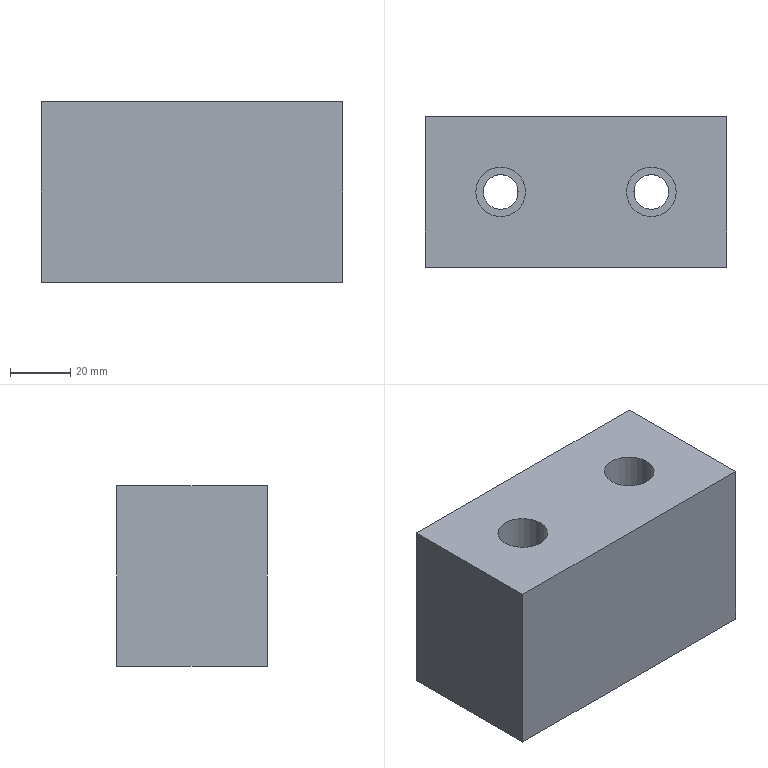Part | NX | features solid 2 | 1 solid | 12 faces | box 100 x 50 x 60 mm | volume 284237 mm3 | plane 8 | cylinder 4 | commonest cylinder face diameters 11.5 x2 16.5 x2
STEP:
#1=CARTESIAN_POINT('',(-1315.,-382.5,-70.));
#2=VERTEX_POINT('',#1);
#3=CARTESIAN_POINT('',(-1315.,-382.5,-130.));
#4=VERTEX_POINT('',#3);
#5=CARTESIAN_POINT('',(-1315.,-382.5,-140.));
#6=DIRECTION('',(0.,0.,1.));
#7=VECTOR('',#6,1000.);
#8=LINE('',#5,#7);
#9=EDGE_CURVE('',#2,#4,#8,.F.);
#10=ORIENTED_EDGE('',*,*,#9,.F.);
#11=CARTESIAN_POINT('',(-1415.,-382.5,-70.));
#12=VERTEX_POINT('',#11);
#13=CARTESIAN_POINT('',(-1325.,-382.5,-70.));
#14=DIRECTION('',(-1.,0.,0.));
#15=VECTOR('',#14,1000.);
#16=LINE('',#13,#15);
#17=EDGE_CURVE('',#2,#12,#16,.T.);
#18=ORIENTED_EDGE('',*,*,#17,.T.);
#19=CARTESIAN_POINT('',(-1415.,-382.5,-130.));
#20=VERTEX_POINT('',#19);
#21=CARTESIAN_POINT('',(-1415.,-382.5,-140.));
#22=DIRECTION('',(0.,0.,-1.));
#23=VECTOR('',#22,1000.);
#24=LINE('',#21,#23);
#25=EDGE_CURVE('',#12,#20,#24,.T.);
#26=ORIENTED_EDGE('',*,*,#25,.T.);
#27=CARTESIAN_POINT('',(-1325.,-382.5,-130.));
#28=DIRECTION('',(-1.,0.,0.));
#29=VECTOR('',#28,1000.);
#30=LINE('',#27,#29);
#31=EDGE_CURVE('',#4,#20,#30,.T.);
#32=ORIENTED_EDGE('',*,*,#31,.F.);
#33=EDGE_LOOP('',(#10,#18,#26,#32));
#34=FACE_BOUND('',#33,.T.);
#35=CARTESIAN_POINT('',(-1325.,-382.5,-140.));
#36=DIRECTION('',(0.,-1.,0.));
#37=DIRECTION('',(-1.,0.,0.));
#38=AXIS2_PLACEMENT_3D('',#35,#36,#37);
#39=PLANE('',#38);
#40=ADVANCED_FACE('',(#34),#39,.T.);
#41=ORIENTED_EDGE('',*,*,#25,.F.);
#42=CARTESIAN_POINT('',(-1415.,-332.5,-70.));
#43=VERTEX_POINT('',#42);
#44=CARTESIAN_POINT('',(-1415.,-367.5,-70.));
#45=DIRECTION('',(0.,1.,0.));
#46=VECTOR('',#45,1000.);
#47=LINE('',#44,#46);
#48=EDGE_CURVE('',#12,#43,#47,.T.);
#49=ORIENTED_EDGE('',*,*,#48,.T.);
#50=CARTESIAN_POINT('',(-1415.,-332.5,-130.));
#51=VERTEX_POINT('',#50);
#52=CARTESIAN_POINT('',(-1415.,-332.5,-140.));
#53=DIRECTION('',(0.,0.,1.));
#54=VECTOR('',#53,1000.);
#55=LINE('',#52,#54);
#56=EDGE_CURVE('',#43,#51,#55,.F.);
#57=ORIENTED_EDGE('',*,*,#56,.T.);
#58=CARTESIAN_POINT('',(-1415.,-367.5,-130.));
#59=DIRECTION('',(0.,1.,0.));
#60=VECTOR('',#59,1000.);
#61=LINE('',#58,#60);
#62=EDGE_CURVE('',#20,#51,#61,.T.);
#63=ORIENTED_EDGE('',*,*,#62,.F.);
#64=EDGE_LOOP('',(#41,#49,#57,#63));
#65=FACE_BOUND('',#64,.T.);
#66=CARTESIAN_POINT('',(-1415.,-367.5,-140.));
#67=DIRECTION('',(-1.,0.,0.));
#68=DIRECTION('',(0.,1.,0.));
#69=AXIS2_PLACEMENT_3D('',#66,#67,#68);
#70=PLANE('',#69);
#71=ADVANCED_FACE('',(#65),#70,.T.);
#72=ORIENTED_EDGE('',*,*,#56,.F.);
#73=CARTESIAN_POINT('',(-1315.,-332.5,-70.));
#74=VERTEX_POINT('',#73);
#75=CARTESIAN_POINT('',(-1325.,-332.5,-70.));
#76=DIRECTION('',(1.,0.,0.));
#77=VECTOR('',#76,1000.);
#78=LINE('',#75,#77);
#79=EDGE_CURVE('',#74,#43,#78,.F.);
#80=ORIENTED_EDGE('',*,*,#79,.F.);
#81=CARTESIAN_POINT('',(-1315.,-332.5,-130.));
#82=VERTEX_POINT('',#81);
#83=CARTESIAN_POINT('',(-1315.,-332.5,-140.));
#84=DIRECTION('',(0.,0.,-1.));
#85=VECTOR('',#84,1000.);
#86=LINE('',#83,#85);
#87=EDGE_CURVE('',#74,#82,#86,.T.);
#88=ORIENTED_EDGE('',*,*,#87,.T.);
#89=CARTESIAN_POINT('',(-1325.,-332.5,-130.));
#90=DIRECTION('',(1.,0.,0.));
#91=VECTOR('',#90,1000.);
#92=LINE('',#89,#91);
#93=EDGE_CURVE('',#82,#51,#92,.F.);
#94=ORIENTED_EDGE('',*,*,#93,.T.);
#95=EDGE_LOOP('',(#72,#80,#88,#94));
#96=FACE_BOUND('',#95,.T.);
#97=CARTESIAN_POINT('',(-1325.,-332.5,-140.));
#98=DIRECTION('',(0.,-1.,0.));
#99=DIRECTION('',(-1.,0.,0.));
#100=AXIS2_PLACEMENT_3D('',#97,#98,#99);
#101=PLANE('',#100);
#102=ADVANCED_FACE('',(#96),#101,.F.);
#103=CARTESIAN_POINT('',(-1315.,-367.5,-70.));
#104=DIRECTION('',(0.,-1.,0.));
#105=VECTOR('',#104,1000.);
#106=LINE('',#103,#105);
#107=EDGE_CURVE('',#2,#74,#106,.F.);
#108=ORIENTED_EDGE('',*,*,#107,.F.);
#109=ORIENTED_EDGE('',*,*,#9,.T.);
#110=CARTESIAN_POINT('',(-1315.,-367.5,-130.));
#111=DIRECTION('',(0.,-1.,0.));
#112=VECTOR('',#111,1000.);
#113=LINE('',#110,#112);
#114=EDGE_CURVE('',#4,#82,#113,.F.);
#115=ORIENTED_EDGE('',*,*,#114,.T.);
#116=ORIENTED_EDGE('',*,*,#87,.F.);
#117=EDGE_LOOP('',(#108,#109,#115,#116));
#118=FACE_BOUND('',#117,.T.);
#119=CARTESIAN_POINT('',(-1315.,-367.5,-140.));
#120=DIRECTION('',(-1.,0.,0.));
#121=DIRECTION('',(0.,1.,0.));
#122=AXIS2_PLACEMENT_3D('',#119,#120,#121);
#123=PLANE('',#122);
#124=ADVANCED_FACE('',(#118),#123,.F.);
#125=CARTESIAN_POINT('',(-1384.25,-357.5,-130.));
#126=VERTEX_POINT('',#125);
#127=CARTESIAN_POINT('',(-1390.,-357.5,-130.));
#128=DIRECTION('',(0.,0.,-1.));
#129=DIRECTION('',(1.,0.,0.));
#130=AXIS2_PLACEMENT_3D('',#127,#128,#129);
#131=CIRCLE('',#130,5.75);
#132=EDGE_CURVE('',#126,#126,#131,.T.);
#133=ORIENTED_EDGE('',*,*,#132,.F.);
#134=EDGE_LOOP('',(#133));
#135=FACE_BOUND('',#134,.T.);
#136=CARTESIAN_POINT('',(-1334.25,-357.5,-130.));
#137=VERTEX_POINT('',#136);
#138=CARTESIAN_POINT('',(-1340.,-357.5,-130.));
#139=DIRECTION('',(0.,0.,-1.));
#140=DIRECTION('',(1.,0.,0.));
#141=AXIS2_PLACEMENT_3D('',#138,#139,#140);
#142=CIRCLE('',#141,5.75);
#143=EDGE_CURVE('',#137,#137,#142,.T.);
#144=ORIENTED_EDGE('',*,*,#143,.F.);
#145=EDGE_LOOP('',(#144));
#146=FACE_BOUND('',#145,.T.);
#147=ORIENTED_EDGE('',*,*,#93,.F.);
#148=ORIENTED_EDGE('',*,*,#114,.F.);
#149=ORIENTED_EDGE('',*,*,#31,.T.);
#150=ORIENTED_EDGE('',*,*,#62,.T.);
#151=EDGE_LOOP('',(#147,#148,#149,#150));
#152=FACE_BOUND('',#151,.T.);
#153=CARTESIAN_POINT('',(-1325.,-367.5,-130.));
#154=DIRECTION('',(0.,0.,-1.));
#155=DIRECTION('',(-1.,0.,0.));
#156=AXIS2_PLACEMENT_3D('',#153,#154,#155);
#157=PLANE('',#156);
#158=ADVANCED_FACE('',(#135,#146,#152),#157,.T.);
#159=CARTESIAN_POINT('',(-1348.25,-357.5,-70.));
#160=VERTEX_POINT('',#159);
#161=CARTESIAN_POINT('',(-1340.,-357.5,-70.));
#162=DIRECTION('',(0.,0.,1.));
#163=DIRECTION('',(-1.,0.,0.));
#164=AXIS2_PLACEMENT_3D('',#161,#162,#163);
#165=CIRCLE('',#164,8.25);
#166=EDGE_CURVE('',#160,#160,#165,.T.);
#167=ORIENTED_EDGE('',*,*,#166,.F.);
#168=EDGE_LOOP('',(#167));
#169=FACE_BOUND('',#168,.T.);
#170=CARTESIAN_POINT('',(-1398.25,-357.5,-70.));
#171=VERTEX_POINT('',#170);
#172=CARTESIAN_POINT('',(-1390.,-357.5,-70.));
#173=DIRECTION('',(0.,0.,1.));
#174=DIRECTION('',(-1.,0.,0.));
#175=AXIS2_PLACEMENT_3D('',#172,#173,#174);
#176=CIRCLE('',#175,8.25);
#177=EDGE_CURVE('',#171,#171,#176,.T.);
#178=ORIENTED_EDGE('',*,*,#177,.F.);
#179=EDGE_LOOP('',(#178));
#180=FACE_BOUND('',#179,.T.);
#181=ORIENTED_EDGE('',*,*,#79,.T.);
#182=ORIENTED_EDGE('',*,*,#48,.F.);
#183=ORIENTED_EDGE('',*,*,#17,.F.);
#184=ORIENTED_EDGE('',*,*,#107,.T.);
#185=EDGE_LOOP('',(#181,#182,#183,#184));
#186=FACE_BOUND('',#185,.T.);
#187=CARTESIAN_POINT('',(-1325.,-367.5,-70.));
#188=DIRECTION('',(0.,0.,-1.));
#189=DIRECTION('',(-1.,0.,0.));
#190=AXIS2_PLACEMENT_3D('',#187,#188,#189);
#191=PLANE('',#190);
#192=ADVANCED_FACE('',(#169,#180,#186),#191,.F.);
#193=CARTESIAN_POINT('',(-1398.25,-357.5,-85.));
#194=VERTEX_POINT('',#193);
#195=CARTESIAN_POINT('',(-1390.,-357.5,-85.));
#196=DIRECTION('',(0.,0.,1.));
#197=DIRECTION('',(-1.,0.,0.));
#198=AXIS2_PLACEMENT_3D('',#195,#196,#197);
#199=CIRCLE('',#198,8.25);
#200=EDGE_CURVE('',#194,#194,#199,.T.);
#201=ORIENTED_EDGE('',*,*,#200,.F.);
#202=EDGE_LOOP('',(#201));
#203=FACE_BOUND('',#202,.T.);
#204=ORIENTED_EDGE('',*,*,#177,.T.);
#205=EDGE_LOOP('',(#204));
#206=FACE_BOUND('',#205,.T.);
#207=CARTESIAN_POINT('',(-1390.,-357.5,-85.));
#208=DIRECTION('',(0.,0.,1.));
#209=DIRECTION('',(-1.,0.,0.));
#210=AXIS2_PLACEMENT_3D('',#207,#208,#209);
#211=CYLINDRICAL_SURFACE('',#210,8.25);
#212=ADVANCED_FACE('',(#203,#206),#211,.F.);
#213=CARTESIAN_POINT('',(-1395.75,-357.5,-85.));
#214=VERTEX_POINT('',#213);
#215=CARTESIAN_POINT('',(-1390.,-357.5,-85.));
#216=DIRECTION('',(0.,0.,1.));
#217=DIRECTION('',(-1.,0.,0.));
#218=AXIS2_PLACEMENT_3D('',#215,#216,#217);
#219=CIRCLE('',#218,5.75);
#220=EDGE_CURVE('',#214,#214,#219,.T.);
#221=ORIENTED_EDGE('',*,*,#220,.F.);
#222=EDGE_LOOP('',(#221));
#223=FACE_BOUND('',#222,.T.);
#224=ORIENTED_EDGE('',*,*,#200,.T.);
#225=EDGE_LOOP('',(#224));
#226=FACE_BOUND('',#225,.T.);
#227=CARTESIAN_POINT('',(-1390.,-352.5,-85.));
#228=DIRECTION('',(0.,0.,1.));
#229=DIRECTION('',(-1.,0.,0.));
#230=AXIS2_PLACEMENT_3D('',#227,#228,#229);
#231=PLANE('',#230);
#232=ADVANCED_FACE('',(#223,#226),#231,.T.);
#233=CARTESIAN_POINT('',(-1348.25,-357.5,-85.));
#234=VERTEX_POINT('',#233);
#235=CARTESIAN_POINT('',(-1340.,-357.5,-85.));
#236=DIRECTION('',(0.,0.,1.));
#237=DIRECTION('',(-1.,0.,0.));
#238=AXIS2_PLACEMENT_3D('',#235,#236,#237);
#239=CIRCLE('',#238,8.25);
#240=EDGE_CURVE('',#234,#234,#239,.T.);
#241=ORIENTED_EDGE('',*,*,#240,.F.);
#242=EDGE_LOOP('',(#241));
#243=FACE_BOUND('',#242,.T.);
#244=ORIENTED_EDGE('',*,*,#166,.T.);
#245=EDGE_LOOP('',(#244));
#246=FACE_BOUND('',#245,.T.);
#247=CARTESIAN_POINT('',(-1340.,-357.5,-85.));
#248=DIRECTION('',(0.,0.,1.));
#249=DIRECTION('',(-1.,0.,0.));
#250=AXIS2_PLACEMENT_3D('',#247,#248,#249);
#251=CYLINDRICAL_SURFACE('',#250,8.25);
#252=ADVANCED_FACE('',(#243,#246),#251,.F.);
#253=CARTESIAN_POINT('',(-1345.75,-357.5,-85.));
#254=VERTEX_POINT('',#253);
#255=CARTESIAN_POINT('',(-1340.,-357.5,-85.));
#256=DIRECTION('',(0.,0.,1.));
#257=DIRECTION('',(-1.,0.,0.));
#258=AXIS2_PLACEMENT_3D('',#255,#256,#257);
#259=CIRCLE('',#258,5.75);
#260=EDGE_CURVE('',#254,#254,#259,.T.);
#261=ORIENTED_EDGE('',*,*,#260,.F.);
#262=EDGE_LOOP('',(#261));
#263=FACE_BOUND('',#262,.T.);
#264=ORIENTED_EDGE('',*,*,#240,.T.);
#265=EDGE_LOOP('',(#264));
#266=FACE_BOUND('',#265,.T.);
#267=CARTESIAN_POINT('',(-1340.,-352.5,-85.));
#268=DIRECTION('',(0.,0.,1.));
#269=DIRECTION('',(-1.,0.,0.));
#270=AXIS2_PLACEMENT_3D('',#267,#268,#269);
#271=PLANE('',#270);
#272=ADVANCED_FACE('',(#263,#266),#271,.T.);
#273=ORIENTED_EDGE('',*,*,#143,.T.);
#274=EDGE_LOOP('',(#273));
#275=FACE_BOUND('',#274,.T.);
#276=ORIENTED_EDGE('',*,*,#260,.T.);
#277=EDGE_LOOP('',(#276));
#278=FACE_BOUND('',#277,.T.);
#279=CARTESIAN_POINT('',(-1340.,-357.5,-220.));
#280=DIRECTION('',(0.,0.,1.));
#281=DIRECTION('',(-1.,0.,0.));
#282=AXIS2_PLACEMENT_3D('',#279,#280,#281);
#283=CYLINDRICAL_SURFACE('',#282,5.75);
#284=ADVANCED_FACE('',(#275,#278),#283,.F.);
#285=ORIENTED_EDGE('',*,*,#132,.T.);
#286=EDGE_LOOP('',(#285));
#287=FACE_BOUND('',#286,.T.);
#288=ORIENTED_EDGE('',*,*,#220,.T.);
#289=EDGE_LOOP('',(#288));
#290=FACE_BOUND('',#289,.T.);
#291=CARTESIAN_POINT('',(-1390.,-357.5,-220.));
#292=DIRECTION('',(0.,0.,1.));
#293=DIRECTION('',(-1.,0.,0.));
#294=AXIS2_PLACEMENT_3D('',#291,#292,#293);
#295=CYLINDRICAL_SURFACE('',#294,5.75);
#296=ADVANCED_FACE('',(#287,#290),#295,.F.);
#297=CLOSED_SHELL('',(#40,#71,#102,#124,#158,#192,#212,#232,#252,#272,#284,#296));
#298=MANIFOLD_SOLID_BREP('',#297);
#299=(LENGTH_UNIT()NAMED_UNIT(*)SI_UNIT(.MILLI.,.METRE.));
#300=UNCERTAINTY_MEASURE_WITH_UNIT(LENGTH_MEASURE(0.00001),#299,'','');
#301=(NAMED_UNIT(*)PLANE_ANGLE_UNIT()SI_UNIT($,.RADIAN.));
#302=(NAMED_UNIT(*)SI_UNIT($,.STERADIAN.)SOLID_ANGLE_UNIT());
#303=(GEOMETRIC_REPRESENTATION_CONTEXT(3)GLOBAL_UNCERTAINTY_ASSIGNED_CONTEXT((#300))GLOBAL_UNIT_ASSIGNED_CONTEXT((#299,#301,#302))REPRESENTATION_CONTEXT('',''));
#304=ADVANCED_BREP_SHAPE_REPRESENTATION('',(#298),#303);